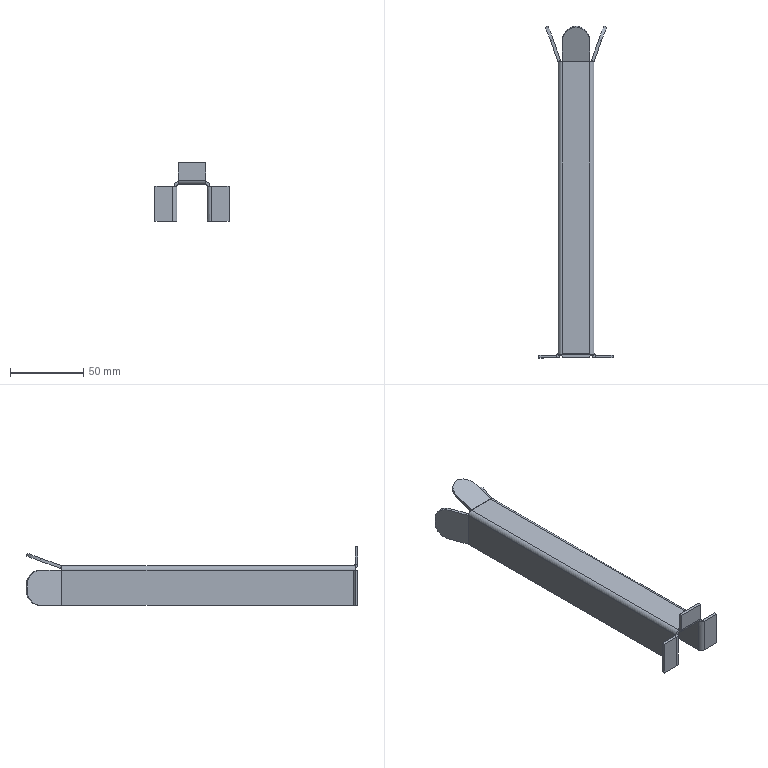Part | SolidWorks | features EdgeFlange 3, Fillet 1, FlatPattern 1, SMBaseFlange 1, SheetMetal 1 | 1 solid | 83 faces | box 50.5 x 226.176 x 40 mm | volume 34108 mm3 | plane 61 | cylinder 22 | commonest cylinder face diameters 2 x8 6 x8 20 x6